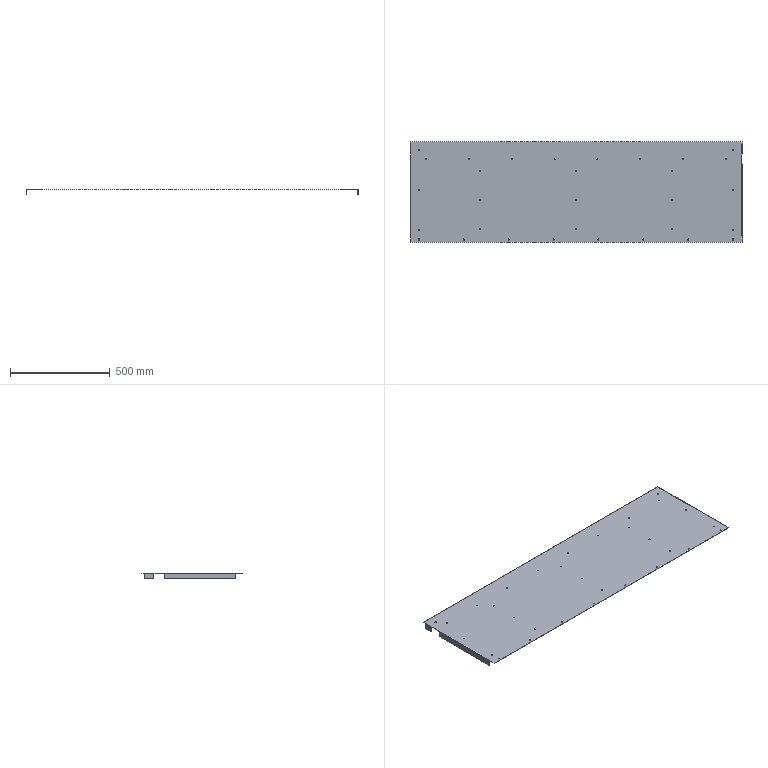Part | STEP file | TS-S33 | 1 solid | 118 faces | box 1665 x 502.5 x 30 mm | volume 1030433 mm3 | cylinder 78 | plane 40 | commonest cylinder face diameters 5.4 x62 10 x8 0.4 x4 2.8 x4